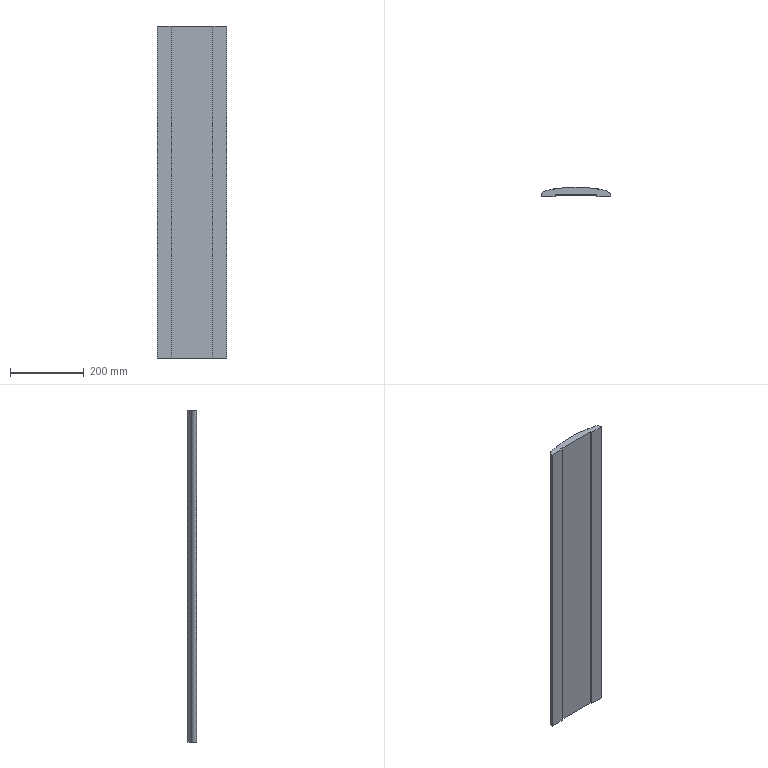Part | SolidWorks | features Extrusion 1, Fillet 1 | 1 solid | 31 faces | box 188.037 x 25 x 900 mm | volume 2969495 mm3 | cylinder 24 | plane 7 | commonest cylinder face diameters 0.2 x8 0.6 x6 661 x5 28 x3 0.4 x2
STEP:
#1=CARTESIAN_POINT('',(-94.018,0.7177,450.));
#2=VERTEX_POINT('',#1);
#3=CARTESIAN_POINT('',(-94.012,0.2909,450.));
#4=VERTEX_POINT('',#3);
#5=CARTESIAN_POINT('',(-80.018,0.7177,450.));
#6=DIRECTION('',(0.,0.,1.));
#7=DIRECTION('',(1.,0.,0.));
#8=AXIS2_PLACEMENT_3D('',#5,#6,#7);
#9=CIRCLE('',#8,14.);
#10=EDGE_CURVE('',#2,#4,#9,.T.);
#11=ORIENTED_EDGE('',*,*,#10,.F.);
#12=CARTESIAN_POINT('',(-94.018,0.7177,-450.));
#13=VERTEX_POINT('',#12);
#14=CARTESIAN_POINT('',(-94.018,0.7177,450.));
#15=DIRECTION('',(0.,0.,-1.));
#16=VECTOR('',#15,1000.);
#17=LINE('',#14,#16);
#18=EDGE_CURVE('',#2,#13,#17,.T.);
#19=ORIENTED_EDGE('',*,*,#18,.T.);
#20=CARTESIAN_POINT('',(-94.012,0.2909,-450.));
#21=VERTEX_POINT('',#20);
#22=CARTESIAN_POINT('',(-80.018,0.7177,-450.));
#23=DIRECTION('',(0.,0.,1.));
#24=DIRECTION('',(1.,0.,0.));
#25=AXIS2_PLACEMENT_3D('',#22,#23,#24);
#26=CIRCLE('',#25,14.);
#27=EDGE_CURVE('',#13,#21,#26,.T.);
#28=ORIENTED_EDGE('',*,*,#27,.T.);
#29=CARTESIAN_POINT('',(-94.012,0.2909,450.));
#30=DIRECTION('',(0.,0.,1.));
#31=VECTOR('',#30,1000.);
#32=LINE('',#29,#31);
#33=EDGE_CURVE('',#21,#4,#32,.T.);
#34=ORIENTED_EDGE('',*,*,#33,.T.);
#35=EDGE_LOOP('',(#11,#19,#28,#34));
#36=FACE_OUTER_BOUND('',#35,.T.);
#37=CARTESIAN_POINT('',(-80.018,0.7177,450.));
#38=DIRECTION('',(0.,0.,-1.));
#39=DIRECTION('',(-1.,0.,0.));
#40=AXIS2_PLACEMENT_3D('',#37,#38,#39);
#41=CYLINDRICAL_SURFACE('',#40,14.);
#42=ADVANCED_FACE('',(#36),#41,.T.);
#43=ORIENTED_EDGE('',*,*,#18,.F.);
#44=CARTESIAN_POINT('',(-83.558,14.263,450.));
#45=VERTEX_POINT('',#44);
#46=CARTESIAN_POINT('',(-80.018,0.7177,450.));
#47=DIRECTION('',(0.,0.,1.));
#48=DIRECTION('',(1.,0.,0.));
#49=AXIS2_PLACEMENT_3D('',#46,#47,#48);
#50=CIRCLE('',#49,14.);
#51=EDGE_CURVE('',#45,#2,#50,.T.);
#52=ORIENTED_EDGE('',*,*,#51,.F.);
#53=CARTESIAN_POINT('',(-83.558,14.263,-450.));
#54=VERTEX_POINT('',#53);
#55=CARTESIAN_POINT('',(-83.558,14.263,450.));
#56=DIRECTION('',(0.,0.,-1.));
#57=VECTOR('',#56,1000.);
#58=LINE('',#55,#57);
#59=EDGE_CURVE('',#45,#54,#58,.T.);
#60=ORIENTED_EDGE('',*,*,#59,.T.);
#61=CARTESIAN_POINT('',(-80.018,0.7177,-450.));
#62=DIRECTION('',(0.,0.,1.));
#63=DIRECTION('',(1.,0.,0.));
#64=AXIS2_PLACEMENT_3D('',#61,#62,#63);
#65=CIRCLE('',#64,14.);
#66=EDGE_CURVE('',#54,#13,#65,.T.);
#67=ORIENTED_EDGE('',*,*,#66,.T.);
#68=EDGE_LOOP('',(#43,#52,#60,#67));
#69=FACE_OUTER_BOUND('',#68,.T.);
#70=CARTESIAN_POINT('',(-80.018,0.7177,450.));
#71=DIRECTION('',(0.,0.,-1.));
#72=DIRECTION('',(-1.,0.,0.));
#73=AXIS2_PLACEMENT_3D('',#70,#71,#72);
#74=CYLINDRICAL_SURFACE('',#73,14.);
#75=ADVANCED_FACE('',(#69),#74,.T.);
#76=CARTESIAN_POINT('',(-93.712,0.,450.));
#77=VERTEX_POINT('',#76);
#78=CARTESIAN_POINT('',(-56.7,0.,450.));
#79=VERTEX_POINT('',#78);
#80=CARTESIAN_POINT('',(-56.7,0.,450.));
#81=DIRECTION('',(1.,0.,0.));
#82=VECTOR('',#81,1000.);
#83=LINE('',#80,#82);
#84=EDGE_CURVE('',#77,#79,#83,.T.);
#85=ORIENTED_EDGE('',*,*,#84,.F.);
#86=CARTESIAN_POINT('',(-93.712,0.,-450.));
#87=VERTEX_POINT('',#86);
#88=CARTESIAN_POINT('',(-93.712,0.,450.));
#89=DIRECTION('',(0.,0.,-1.));
#90=VECTOR('',#89,1000.);
#91=LINE('',#88,#90);
#92=EDGE_CURVE('',#77,#87,#91,.T.);
#93=ORIENTED_EDGE('',*,*,#92,.T.);
#94=CARTESIAN_POINT('',(-56.7,0.,-450.));
#95=VERTEX_POINT('',#94);
#96=CARTESIAN_POINT('',(-56.7,0.,-450.));
#97=DIRECTION('',(1.,0.,0.));
#98=VECTOR('',#97,1000.);
#99=LINE('',#96,#98);
#100=EDGE_CURVE('',#87,#95,#99,.T.);
#101=ORIENTED_EDGE('',*,*,#100,.T.);
#102=CARTESIAN_POINT('',(-56.7,0.,450.));
#103=DIRECTION('',(0.,0.,-1.));
#104=VECTOR('',#103,1000.);
#105=LINE('',#102,#104);
#106=EDGE_CURVE('',#79,#95,#105,.T.);
#107=ORIENTED_EDGE('',*,*,#106,.F.);
#108=EDGE_LOOP('',(#85,#93,#101,#107));
#109=FACE_OUTER_BOUND('',#108,.T.);
#110=CARTESIAN_POINT('',(-56.7,0.,450.));
#111=DIRECTION('',(0.,1.,0.));
#112=DIRECTION('',(-1.,0.,0.));
#113=AXIS2_PLACEMENT_3D('',#110,#111,#112);
#114=PLANE('',#113);
#115=ADVANCED_FACE('',(#109),#114,.F.);
#116=CARTESIAN_POINT('',(-56.5,0.2,-450.));
#117=VERTEX_POINT('',#116);
#118=CARTESIAN_POINT('',(-56.7,0.2,-450.));
#119=DIRECTION('',(0.,0.,1.));
#120=DIRECTION('',(-1.,0.,0.));
#121=AXIS2_PLACEMENT_3D('',#118,#119,#120);
#122=CIRCLE('',#121,0.2);
#123=EDGE_CURVE('',#95,#117,#122,.T.);
#124=ORIENTED_EDGE('',*,*,#123,.T.);
#125=CARTESIAN_POINT('',(-56.5,0.2,450.));
#126=VERTEX_POINT('',#125);
#127=CARTESIAN_POINT('',(-56.5,0.2,450.));
#128=DIRECTION('',(0.,0.,-1.));
#129=VECTOR('',#128,1000.);
#130=LINE('',#127,#129);
#131=EDGE_CURVE('',#126,#117,#130,.T.);
#132=ORIENTED_EDGE('',*,*,#131,.F.);
#133=CARTESIAN_POINT('',(-56.7,0.2,450.));
#134=DIRECTION('',(0.,0.,1.));
#135=DIRECTION('',(-1.,0.,0.));
#136=AXIS2_PLACEMENT_3D('',#133,#134,#135);
#137=CIRCLE('',#136,0.2);
#138=EDGE_CURVE('',#79,#126,#137,.T.);
#139=ORIENTED_EDGE('',*,*,#138,.F.);
#140=ORIENTED_EDGE('',*,*,#106,.T.);
#141=EDGE_LOOP('',(#124,#132,#139,#140));
#142=FACE_OUTER_BOUND('',#141,.T.);
#143=CARTESIAN_POINT('',(-56.7,0.2,450.));
#144=DIRECTION('',(0.,0.,-1.));
#145=DIRECTION('',(-1.,0.,0.));
#146=AXIS2_PLACEMENT_3D('',#143,#144,#145);
#147=CYLINDRICAL_SURFACE('',#146,0.2);
#148=ADVANCED_FACE('',(#142),#147,.T.);
#149=CARTESIAN_POINT('',(-56.5,4.5,-450.));
#150=VERTEX_POINT('',#149);
#151=CARTESIAN_POINT('',(-56.5,0.2,-450.));
#152=DIRECTION('',(0.,1.,0.));
#153=VECTOR('',#152,1000.);
#154=LINE('',#151,#153);
#155=EDGE_CURVE('',#117,#150,#154,.T.);
#156=ORIENTED_EDGE('',*,*,#155,.T.);
#157=CARTESIAN_POINT('',(-56.5,4.5,450.));
#158=VERTEX_POINT('',#157);
#159=CARTESIAN_POINT('',(-56.5,4.5,450.));
#160=DIRECTION('',(0.,0.,-1.));
#161=VECTOR('',#160,1000.);
#162=LINE('',#159,#161);
#163=EDGE_CURVE('',#158,#150,#162,.T.);
#164=ORIENTED_EDGE('',*,*,#163,.F.);
#165=CARTESIAN_POINT('',(-56.5,0.2,450.));
#166=DIRECTION('',(0.,1.,0.));
#167=VECTOR('',#166,1000.);
#168=LINE('',#165,#167);
#169=EDGE_CURVE('',#126,#158,#168,.T.);
#170=ORIENTED_EDGE('',*,*,#169,.F.);
#171=ORIENTED_EDGE('',*,*,#131,.T.);
#172=EDGE_LOOP('',(#156,#164,#170,#171));
#173=FACE_OUTER_BOUND('',#172,.T.);
#174=CARTESIAN_POINT('',(-56.5,0.2,450.));
#175=DIRECTION('',(-1.,0.,0.));
#176=DIRECTION('',(0.,-1.,0.));
#177=AXIS2_PLACEMENT_3D('',#174,#175,#176);
#178=PLANE('',#177);
#179=ADVANCED_FACE('',(#173),#178,.F.);
#180=CARTESIAN_POINT('',(56.5,4.5,-450.));
#181=VERTEX_POINT('',#180);
#182=CARTESIAN_POINT('',(-56.5,4.5,-450.));
#183=DIRECTION('',(1.,0.,0.));
#184=VECTOR('',#183,1000.);
#185=LINE('',#182,#184);
#186=EDGE_CURVE('',#150,#181,#185,.T.);
#187=ORIENTED_EDGE('',*,*,#186,.T.);
#188=CARTESIAN_POINT('',(56.5,4.5,450.));
#189=VERTEX_POINT('',#188);
#190=CARTESIAN_POINT('',(56.5,4.5,450.));
#191=DIRECTION('',(0.,0.,-1.));
#192=VECTOR('',#191,1000.);
#193=LINE('',#190,#192);
#194=EDGE_CURVE('',#189,#181,#193,.T.);
#195=ORIENTED_EDGE('',*,*,#194,.F.);
#196=CARTESIAN_POINT('',(-56.5,4.5,450.));
#197=DIRECTION('',(1.,0.,0.));
#198=VECTOR('',#197,1000.);
#199=LINE('',#196,#198);
#200=EDGE_CURVE('',#158,#189,#199,.T.);
#201=ORIENTED_EDGE('',*,*,#200,.F.);
#202=ORIENTED_EDGE('',*,*,#163,.T.);
#203=EDGE_LOOP('',(#187,#195,#201,#202));
#204=FACE_OUTER_BOUND('',#203,.T.);
#205=CARTESIAN_POINT('',(-56.5,4.5,450.));
#206=DIRECTION('',(0.,1.,0.));
#207=DIRECTION('',(-1.,0.,0.));
#208=AXIS2_PLACEMENT_3D('',#205,#206,#207);
#209=PLANE('',#208);
#210=ADVANCED_FACE('',(#204),#209,.F.);
#211=CARTESIAN_POINT('',(56.5,0.2,-450.));
#212=VERTEX_POINT('',#211);
#213=CARTESIAN_POINT('',(56.5,0.2,-450.));
#214=DIRECTION('',(0.,-1.,0.));
#215=VECTOR('',#214,1000.);
#216=LINE('',#213,#215);
#217=EDGE_CURVE('',#181,#212,#216,.T.);
#218=ORIENTED_EDGE('',*,*,#217,.T.);
#219=CARTESIAN_POINT('',(56.5,0.2,450.));
#220=VERTEX_POINT('',#219);
#221=CARTESIAN_POINT('',(56.5,0.2,450.));
#222=DIRECTION('',(0.,0.,-1.));
#223=VECTOR('',#222,1000.);
#224=LINE('',#221,#223);
#225=EDGE_CURVE('',#220,#212,#224,.T.);
#226=ORIENTED_EDGE('',*,*,#225,.F.);
#227=CARTESIAN_POINT('',(56.5,0.2,450.));
#228=DIRECTION('',(0.,-1.,0.));
#229=VECTOR('',#228,1000.);
#230=LINE('',#227,#229);
#231=EDGE_CURVE('',#189,#220,#230,.T.);
#232=ORIENTED_EDGE('',*,*,#231,.F.);
#233=ORIENTED_EDGE('',*,*,#194,.T.);
#234=EDGE_LOOP('',(#218,#226,#232,#233));
#235=FACE_OUTER_BOUND('',#234,.T.);
#236=CARTESIAN_POINT('',(56.5,0.2,450.));
#237=DIRECTION('',(1.,0.,0.));
#238=DIRECTION('',(0.,1.,0.));
#239=AXIS2_PLACEMENT_3D('',#236,#237,#238);
#240=PLANE('',#239);
#241=ADVANCED_FACE('',(#235),#240,.F.);
#242=CARTESIAN_POINT('',(56.7,0.,-450.));
#243=VERTEX_POINT('',#242);
#244=CARTESIAN_POINT('',(56.7,0.2,-450.));
#245=DIRECTION('',(0.,0.,1.));
#246=DIRECTION('',(-1.,0.,0.));
#247=AXIS2_PLACEMENT_3D('',#244,#245,#246);
#248=CIRCLE('',#247,0.2);
#249=EDGE_CURVE('',#212,#243,#248,.T.);
#250=ORIENTED_EDGE('',*,*,#249,.T.);
#251=CARTESIAN_POINT('',(56.7,0.,450.));
#252=VERTEX_POINT('',#251);
#253=CARTESIAN_POINT('',(56.7,0.,450.));
#254=DIRECTION('',(0.,0.,-1.));
#255=VECTOR('',#254,1000.);
#256=LINE('',#253,#255);
#257=EDGE_CURVE('',#252,#243,#256,.T.);
#258=ORIENTED_EDGE('',*,*,#257,.F.);
#259=CARTESIAN_POINT('',(56.7,0.2,450.));
#260=DIRECTION('',(0.,0.,1.));
#261=DIRECTION('',(-1.,0.,0.));
#262=AXIS2_PLACEMENT_3D('',#259,#260,#261);
#263=CIRCLE('',#262,0.2);
#264=EDGE_CURVE('',#220,#252,#263,.T.);
#265=ORIENTED_EDGE('',*,*,#264,.F.);
#266=ORIENTED_EDGE('',*,*,#225,.T.);
#267=EDGE_LOOP('',(#250,#258,#265,#266));
#268=FACE_OUTER_BOUND('',#267,.T.);
#269=CARTESIAN_POINT('',(56.7,0.2,450.));
#270=DIRECTION('',(0.,0.,-1.));
#271=DIRECTION('',(-1.,0.,0.));
#272=AXIS2_PLACEMENT_3D('',#269,#270,#271);
#273=CYLINDRICAL_SURFACE('',#272,0.2);
#274=ADVANCED_FACE('',(#268),#273,.T.);
#275=CARTESIAN_POINT('',(93.712,0.,-450.));
#276=VERTEX_POINT('',#275);
#277=CARTESIAN_POINT('',(94.,0.,-450.));
#278=DIRECTION('',(1.,0.,0.));
#279=VECTOR('',#278,1000.);
#280=LINE('',#277,#279);
#281=EDGE_CURVE('',#243,#276,#280,.T.);
#282=ORIENTED_EDGE('',*,*,#281,.T.);
#283=CARTESIAN_POINT('',(93.712,0.,450.));
#284=VERTEX_POINT('',#283);
#285=CARTESIAN_POINT('',(93.712,0.,450.));
#286=DIRECTION('',(0.,0.,1.));
#287=VECTOR('',#286,1000.);
#288=LINE('',#285,#287);
#289=EDGE_CURVE('',#276,#284,#288,.T.);
#290=ORIENTED_EDGE('',*,*,#289,.T.);
#291=CARTESIAN_POINT('',(94.,0.,450.));
#292=DIRECTION('',(1.,0.,0.));
#293=VECTOR('',#292,1000.);
#294=LINE('',#291,#293);
#295=EDGE_CURVE('',#252,#284,#294,.T.);
#296=ORIENTED_EDGE('',*,*,#295,.F.);
#297=ORIENTED_EDGE('',*,*,#257,.T.);
#298=EDGE_LOOP('',(#282,#290,#296,#297));
#299=FACE_OUTER_BOUND('',#298,.T.);
#300=CARTESIAN_POINT('',(94.,0.,450.));
#301=DIRECTION('',(0.,1.,0.));
#302=DIRECTION('',(-1.,0.,0.));
#303=AXIS2_PLACEMENT_3D('',#300,#301,#302);
#304=PLANE('',#303);
#305=ADVANCED_FACE('',(#299),#304,.F.);
#306=CARTESIAN_POINT('',(94.012,0.2909,450.));
#307=VERTEX_POINT('',#306);
#308=CARTESIAN_POINT('',(83.558,14.263,450.));
#309=VERTEX_POINT('',#308);
#310=CARTESIAN_POINT('',(80.018,0.7177,450.));
#311=DIRECTION('',(0.,0.,1.));
#312=DIRECTION('',(-1.,0.,0.));
#313=AXIS2_PLACEMENT_3D('',#310,#311,#312);
#314=CIRCLE('',#313,14.);
#315=EDGE_CURVE('',#307,#309,#314,.T.);
#316=ORIENTED_EDGE('',*,*,#315,.F.);
#317=CARTESIAN_POINT('',(94.012,0.2909,-450.));
#318=VERTEX_POINT('',#317);
#319=CARTESIAN_POINT('',(94.012,0.2909,450.));
#320=DIRECTION('',(0.,0.,-1.));
#321=VECTOR('',#320,1000.);
#322=LINE('',#319,#321);
#323=EDGE_CURVE('',#307,#318,#322,.T.);
#324=ORIENTED_EDGE('',*,*,#323,.T.);
#325=CARTESIAN_POINT('',(83.558,14.263,-450.));
#326=VERTEX_POINT('',#325);
#327=CARTESIAN_POINT('',(80.018,0.7177,-450.));
#328=DIRECTION('',(0.,0.,1.));
#329=DIRECTION('',(-1.,0.,0.));
#330=AXIS2_PLACEMENT_3D('',#327,#328,#329);
#331=CIRCLE('',#330,14.);
#332=EDGE_CURVE('',#318,#326,#331,.T.);
#333=ORIENTED_EDGE('',*,*,#332,.T.);
#334=CARTESIAN_POINT('',(83.558,14.263,450.));
#335=DIRECTION('',(0.,0.,-1.));
#336=VECTOR('',#335,1000.);
#337=LINE('',#334,#336);
#338=EDGE_CURVE('',#309,#326,#337,.T.);
#339=ORIENTED_EDGE('',*,*,#338,.F.);
#340=EDGE_LOOP('',(#316,#324,#333,#339));
#341=FACE_OUTER_BOUND('',#340,.T.);
#342=CARTESIAN_POINT('',(80.018,0.7177,450.));
#343=DIRECTION('',(0.,0.,-1.));
#344=DIRECTION('',(-1.,0.,0.));
#345=AXIS2_PLACEMENT_3D('',#342,#343,#344);
#346=CYLINDRICAL_SURFACE('',#345,14.);
#347=ADVANCED_FACE('',(#341),#346,.T.);
#348=CARTESIAN_POINT('',(60.381,19.438,-450.));
#349=VERTEX_POINT('',#348);
#350=CARTESIAN_POINT('',(0.,-305.5,-450.));
#351=DIRECTION('',(0.,0.,1.));
#352=DIRECTION('',(1.,0.,0.));
#353=AXIS2_PLACEMENT_3D('',#350,#351,#352);
#354=CIRCLE('',#353,330.5);
#355=EDGE_CURVE('',#326,#349,#354,.T.);
#356=ORIENTED_EDGE('',*,*,#355,.T.);
#357=CARTESIAN_POINT('',(60.381,19.438,450.));
#358=VERTEX_POINT('',#357);
#359=CARTESIAN_POINT('',(60.381,19.438,450.));
#360=DIRECTION('',(0.,0.,-1.));
#361=VECTOR('',#360,1000.);
#362=LINE('',#359,#361);
#363=EDGE_CURVE('',#358,#349,#362,.T.);
#364=ORIENTED_EDGE('',*,*,#363,.F.);
#365=CARTESIAN_POINT('',(0.,-305.5,450.));
#366=DIRECTION('',(0.,0.,1.));
#367=DIRECTION('',(1.,0.,0.));
#368=AXIS2_PLACEMENT_3D('',#365,#366,#367);
#369=CIRCLE('',#368,330.5);
#370=EDGE_CURVE('',#309,#358,#369,.T.);
#371=ORIENTED_EDGE('',*,*,#370,.F.);
#372=ORIENTED_EDGE('',*,*,#338,.T.);
#373=EDGE_LOOP('',(#356,#364,#371,#372));
#374=FACE_OUTER_BOUND('',#373,.T.);
#375=CARTESIAN_POINT('',(0.,-305.5,450.));
#376=DIRECTION('',(0.,0.,-1.));
#377=DIRECTION('',(-1.,0.,0.));
#378=AXIS2_PLACEMENT_3D('',#375,#376,#377);
#379=CYLINDRICAL_SURFACE('',#378,330.5);
#380=ADVANCED_FACE('',(#374),#379,.T.);
#381=CARTESIAN_POINT('',(60.272,19.381,-450.));
#382=VERTEX_POINT('',#381);
#383=CARTESIAN_POINT('',(60.363,19.339,-450.));
#384=DIRECTION('',(0.,0.,1.));
#385=DIRECTION('',(1.,0.,0.));
#386=AXIS2_PLACEMENT_3D('',#383,#384,#385);
#387=CIRCLE('',#386,0.1);
#388=EDGE_CURVE('',#349,#382,#387,.T.);
#389=ORIENTED_EDGE('',*,*,#388,.T.);
#390=CARTESIAN_POINT('',(60.272,19.381,450.));
#391=VERTEX_POINT('',#390);
#392=CARTESIAN_POINT('',(60.272,19.381,450.));
#393=DIRECTION('',(0.,0.,-1.));
#394=VECTOR('',#393,1000.);
#395=LINE('',#392,#394);
#396=EDGE_CURVE('',#391,#382,#395,.T.);
#397=ORIENTED_EDGE('',*,*,#396,.F.);
#398=CARTESIAN_POINT('',(60.363,19.339,450.));
#399=DIRECTION('',(0.,0.,1.));
#400=DIRECTION('',(1.,0.,0.));
#401=AXIS2_PLACEMENT_3D('',#398,#399,#400);
#402=CIRCLE('',#401,0.1);
#403=EDGE_CURVE('',#358,#391,#402,.T.);
#404=ORIENTED_EDGE('',*,*,#403,.F.);
#405=ORIENTED_EDGE('',*,*,#363,.T.);
#406=EDGE_LOOP('',(#389,#397,#404,#405));
#407=FACE_OUTER_BOUND('',#406,.T.);
#408=CARTESIAN_POINT('',(60.363,19.339,450.));
#409=DIRECTION('',(0.,0.,-1.));
#410=DIRECTION('',(-1.,0.,0.));
#411=AXIS2_PLACEMENT_3D('',#408,#409,#410);
#412=CYLINDRICAL_SURFACE('',#411,0.1);
#413=ADVANCED_FACE('',(#407),#412,.T.);
#414=CARTESIAN_POINT('',(59.701,19.487,-450.));
#415=VERTEX_POINT('',#414);
#416=CARTESIAN_POINT('',(60.,19.508,-450.));
#417=DIRECTION('',(0.,0.,-1.));
#418=DIRECTION('',(-1.,0.,0.));
#419=AXIS2_PLACEMENT_3D('',#416,#417,#418);
#420=CIRCLE('',#419,0.3);
#421=EDGE_CURVE('',#382,#415,#420,.T.);
#422=ORIENTED_EDGE('',*,*,#421,.T.);
#423=CARTESIAN_POINT('',(59.701,19.487,450.));
#424=VERTEX_POINT('',#423);
#425=CARTESIAN_POINT('',(59.701,19.487,450.));
#426=DIRECTION('',(0.,0.,-1.));
#427=VECTOR('',#426,1000.);
#428=LINE('',#425,#427);
#429=EDGE_CURVE('',#424,#415,#428,.T.);
#430=ORIENTED_EDGE('',*,*,#429,.F.);
#431=CARTESIAN_POINT('',(60.,19.508,450.));
#432=DIRECTION('',(0.,0.,-1.));
#433=DIRECTION('',(-1.,0.,0.));
#434=AXIS2_PLACEMENT_3D('',#431,#432,#433);
#435=CIRCLE('',#434,0.3);
#436=EDGE_CURVE('',#391,#424,#435,.T.);
#437=ORIENTED_EDGE('',*,*,#436,.F.);
#438=ORIENTED_EDGE('',*,*,#396,.T.);
#439=EDGE_LOOP('',(#422,#430,#437,#438));
#440=FACE_OUTER_BOUND('',#439,.T.);
#441=CARTESIAN_POINT('',(60.,19.508,450.));
#442=DIRECTION('',(0.,0.,-1.));
#443=DIRECTION('',(-1.,0.,0.));
#444=AXIS2_PLACEMENT_3D('',#441,#442,#443);
#445=CYLINDRICAL_SURFACE('',#444,0.3);
#446=ADVANCED_FACE('',(#440),#445,.F.);
#447=CARTESIAN_POINT('',(59.619,19.578,-450.));
#448=VERTEX_POINT('',#447);
#449=CARTESIAN_POINT('',(59.601,19.48,-450.));
#450=DIRECTION('',(0.,0.,1.));
#451=DIRECTION('',(1.,0.,0.));
#452=AXIS2_PLACEMENT_3D('',#449,#450,#451);
#453=CIRCLE('',#452,0.1);
#454=EDGE_CURVE('',#415,#448,#453,.T.);
#455=ORIENTED_EDGE('',*,*,#454,.T.);
#456=CARTESIAN_POINT('',(59.619,19.578,450.));
#457=VERTEX_POINT('',#456);
#458=CARTESIAN_POINT('',(59.619,19.578,450.));
#459=DIRECTION('',(0.,0.,-1.));
#460=VECTOR('',#459,1000.);
#461=LINE('',#458,#460);
#462=EDGE_CURVE('',#457,#448,#461,.T.);
#463=ORIENTED_EDGE('',*,*,#462,.F.);
#464=CARTESIAN_POINT('',(59.601,19.48,450.));
#465=DIRECTION('',(0.,0.,1.));
#466=DIRECTION('',(1.,0.,0.));
#467=AXIS2_PLACEMENT_3D('',#464,#465,#466);
#468=CIRCLE('',#467,0.1);
#469=EDGE_CURVE('',#424,#457,#468,.T.);
#470=ORIENTED_EDGE('',*,*,#469,.F.);
#471=ORIENTED_EDGE('',*,*,#429,.T.);
#472=EDGE_LOOP('',(#455,#463,#470,#471));
#473=FACE_OUTER_BOUND('',#472,.T.);
#474=CARTESIAN_POINT('',(59.601,19.48,450.));
#475=DIRECTION('',(0.,0.,-1.));
#476=DIRECTION('',(-1.,0.,0.));
#477=AXIS2_PLACEMENT_3D('',#474,#475,#476);
#478=CYLINDRICAL_SURFACE('',#477,0.1);
#479=ADVANCED_FACE('',(#473),#478,.T.);
#480=CARTESIAN_POINT('',(59.381,19.622,-450.));
#481=VERTEX_POINT('',#480);
#482=CARTESIAN_POINT('',(0.,-305.5,-450.));
#483=DIRECTION('',(0.,0.,1.));
#484=DIRECTION('',(1.,0.,0.));
#485=AXIS2_PLACEMENT_3D('',#482,#483,#484);
#486=CIRCLE('',#485,330.5);
#487=EDGE_CURVE('',#448,#481,#486,.T.);
#488=ORIENTED_EDGE('',*,*,#487,.T.);
#489=CARTESIAN_POINT('',(59.381,19.622,450.));
#490=VERTEX_POINT('',#489);
#491=CARTESIAN_POINT('',(59.381,19.622,450.));
#492=DIRECTION('',(0.,0.,-1.));
#493=VECTOR('',#492,1000.);
#494=LINE('',#491,#493);
#495=EDGE_CURVE('',#490,#481,#494,.T.);
#496=ORIENTED_EDGE('',*,*,#495,.F.);
#497=CARTESIAN_POINT('',(0.,-305.5,450.));
#498=DIRECTION('',(0.,0.,1.));
#499=DIRECTION('',(1.,0.,0.));
#500=AXIS2_PLACEMENT_3D('',#497,#498,#499);
#501=CIRCLE('',#500,330.5);
#502=EDGE_CURVE('',#457,#490,#501,.T.);
#503=ORIENTED_EDGE('',*,*,#502,.F.);
#504=ORIENTED_EDGE('',*,*,#462,.T.);
#505=EDGE_LOOP('',(#488,#496,#503,#504));
#506=FACE_OUTER_BOUND('',#505,.T.);
#507=CARTESIAN_POINT('',(0.,-305.5,450.));
#508=DIRECTION('',(0.,0.,-1.));
#509=DIRECTION('',(-1.,0.,0.));
#510=AXIS2_PLACEMENT_3D('',#507,#508,#509);
#511=CYLINDRICAL_SURFACE('',#510,330.5);
#512=ADVANCED_FACE('',(#506),#511,.T.);
#513=CARTESIAN_POINT('',(59.272,19.565,-450.));
#514=VERTEX_POINT('',#513);
#515=CARTESIAN_POINT('',(59.363,19.523,-450.));
#516=DIRECTION('',(0.,0.,1.));
#517=DIRECTION('',(1.,0.,0.));
#518=AXIS2_PLACEMENT_3D('',#515,#516,#517);
#519=CIRCLE('',#518,0.1);
#520=EDGE_CURVE('',#481,#514,#519,.T.);
#521=ORIENTED_EDGE('',*,*,#520,.T.);
#522=CARTESIAN_POINT('',(59.272,19.565,450.));
#523=VERTEX_POINT('',#522);
#524=CARTESIAN_POINT('',(59.272,19.565,450.));
#525=DIRECTION('',(0.,0.,-1.));
#526=VECTOR('',#525,1000.);
#527=LINE('',#524,#526);
#528=EDGE_CURVE('',#523,#514,#527,.T.);
#529=ORIENTED_EDGE('',*,*,#528,.F.);
#530=CARTESIAN_POINT('',(59.363,19.523,450.));
#531=DIRECTION('',(0.,0.,1.));
#532=DIRECTION('',(1.,0.,0.));
#533=AXIS2_PLACEMENT_3D('',#530,#531,#532);
#534=CIRCLE('',#533,0.1);
#535=EDGE_CURVE('',#490,#523,#534,.T.);
#536=ORIENTED_EDGE('',*,*,#535,.F.);
#537=ORIENTED_EDGE('',*,*,#495,.T.);
#538=EDGE_LOOP('',(#521,#529,#536,#537));
#539=FACE_OUTER_BOUND('',#538,.T.);
#540=CARTESIAN_POINT('',(59.363,19.523,450.));
#541=DIRECTION('',(0.,0.,-1.));
#542=DIRECTION('',(-1.,0.,0.));
#543=AXIS2_PLACEMENT_3D('',#540,#541,#542);
#544=CYLINDRICAL_SURFACE('',#543,0.1);
#545=ADVANCED_FACE('',(#539),#544,.T.);
#546=CARTESIAN_POINT('',(58.701,19.669,-450.));
#547=VERTEX_POINT('',#546);
#548=CARTESIAN_POINT('',(59.,19.691,-450.));
#549=DIRECTION('',(0.,0.,-1.));
#550=DIRECTION('',(-1.,0.,0.));
#551=AXIS2_PLACEMENT_3D('',#548,#549,#550);
#552=CIRCLE('',#551,0.3);
#553=EDGE_CURVE('',#514,#547,#552,.T.);
#554=ORIENTED_EDGE('',*,*,#553,.T.);
#555=CARTESIAN_POINT('',(58.701,19.669,450.));
#556=VERTEX_POINT('',#555);
#557=CARTESIAN_POINT('',(58.701,19.669,450.));
#558=DIRECTION('',(0.,0.,-1.));
#559=VECTOR('',#558,1000.);
#560=LINE('',#557,#559);
#561=EDGE_CURVE('',#556,#547,#560,.T.);
#562=ORIENTED_EDGE('',*,*,#561,.F.);
#563=CARTESIAN_POINT('',(59.,19.691,450.));
#564=DIRECTION('',(0.,0.,-1.));
#565=DIRECTION('',(-1.,0.,0.));
#566=AXIS2_PLACEMENT_3D('',#563,#564,#565);
#567=CIRCLE('',#566,0.3);
#568=EDGE_CURVE('',#523,#556,#567,.T.);
#569=ORIENTED_EDGE('',*,*,#568,.F.);
#570=ORIENTED_EDGE('',*,*,#528,.T.);
#571=EDGE_LOOP('',(#554,#562,#569,#570));
#572=FACE_OUTER_BOUND('',#571,.T.);
#573=CARTESIAN_POINT('',(59.,19.691,450.));
#574=DIRECTION('',(0.,0.,-1.));
#575=DIRECTION('',(-1.,0.,0.));
#576=AXIS2_PLACEMENT_3D('',#573,#574,#575);
#577=CYLINDRICAL_SURFACE('',#576,0.3);
#578=ADVANCED_FACE('',(#572),#577,.F.);
#579=CARTESIAN_POINT('',(58.619,19.76,-450.));
#580=VERTEX_POINT('',#579);
#581=CARTESIAN_POINT('',(58.601,19.662,-450.));
#582=DIRECTION('',(0.,0.,1.));
#583=DIRECTION('',(-1.,0.,0.));
#584=AXIS2_PLACEMENT_3D('',#581,#582,#583);
#585=CIRCLE('',#584,0.1);
#586=EDGE_CURVE('',#547,#580,#585,.T.);
#587=ORIENTED_EDGE('',*,*,#586,.T.);
#588=CARTESIAN_POINT('',(58.619,19.76,450.));
#589=VERTEX_POINT('',#588);
#590=CARTESIAN_POINT('',(58.619,19.76,450.));
#591=DIRECTION('',(0.,0.,-1.));
#592=VECTOR('',#591,1000.);
#593=LINE('',#590,#592);
#594=EDGE_CURVE('',#589,#580,#593,.T.);
#595=ORIENTED_EDGE('',*,*,#594,.F.);
#596=CARTESIAN_POINT('',(58.601,19.662,450.));
#597=DIRECTION('',(0.,0.,1.));
#598=DIRECTION('',(-1.,0.,0.));
#599=AXIS2_PLACEMENT_3D('',#596,#597,#598);
#600=CIRCLE('',#599,0.1);
#601=EDGE_CURVE('',#556,#589,#600,.T.);
#602=ORIENTED_EDGE('',*,*,#601,.F.);
#603=ORIENTED_EDGE('',*,*,#561,.T.);
#604=EDGE_LOOP('',(#587,#595,#602,#603));
#605=FACE_OUTER_BOUND('',#604,.T.);
#606=CARTESIAN_POINT('',(58.601,19.662,450.));
#607=DIRECTION('',(0.,0.,-1.));
#608=DIRECTION('',(-1.,0.,0.));
#609=AXIS2_PLACEMENT_3D('',#606,#607,#608);
#610=CYLINDRICAL_SURFACE('',#609,0.1);
#611=ADVANCED_FACE('',(#605),#610,.T.);
#612=CARTESIAN_POINT('',(-58.619,19.76,-450.));
#613=VERTEX_POINT('',#612);
#614=CARTESIAN_POINT('',(0.,-305.5,-450.));
#615=DIRECTION('',(0.,0.,1.));
#616=DIRECTION('',(1.,0.,0.));
#617=AXIS2_PLACEMENT_3D('',#614,#615,#616);
#618=CIRCLE('',#617,330.5);
#619=EDGE_CURVE('',#580,#613,#618,.T.);
#620=ORIENTED_EDGE('',*,*,#619,.T.);
#621=CARTESIAN_POINT('',(-58.619,19.76,450.));
#622=VERTEX_POINT('',#621);
#623=CARTESIAN_POINT('',(-58.619,19.76,450.));
#624=DIRECTION('',(0.,0.,-1.));
#625=VECTOR('',#624,1000.);
#626=LINE('',#623,#625);
#627=EDGE_CURVE('',#622,#613,#626,.T.);
#628=ORIENTED_EDGE('',*,*,#627,.F.);
#629=CARTESIAN_POINT('',(0.,-305.5,450.));
#630=DIRECTION('',(0.,0.,1.));
#631=DIRECTION('',(1.,0.,0.));
#632=AXIS2_PLACEMENT_3D('',#629,#630,#631);
#633=CIRCLE('',#632,330.5);
#634=EDGE_CURVE('',#589,#622,#633,.T.);
#635=ORIENTED_EDGE('',*,*,#634,.F.);
#636=ORIENTED_EDGE('',*,*,#594,.T.);
#637=EDGE_LOOP('',(#620,#628,#635,#636));
#638=FACE_OUTER_BOUND('',#637,.T.);
#639=CARTESIAN_POINT('',(0.,-305.5,450.));
#640=DIRECTION('',(0.,0.,-1.));
#641=DIRECTION('',(-1.,0.,0.));
#642=AXIS2_PLACEMENT_3D('',#639,#640,#641);
#643=CYLINDRICAL_SURFACE('',#642,330.5);
#644=ADVANCED_FACE('',(#638),#643,.T.);
#645=CARTESIAN_POINT('',(-58.701,19.669,-450.));
#646=VERTEX_POINT('',#645);
#647=CARTESIAN_POINT('',(-58.601,19.662,-450.));
#648=DIRECTION('',(0.,0.,1.));
#649=DIRECTION('',(-1.,0.,0.));
#650=AXIS2_PLACEMENT_3D('',#647,#648,#649);
#651=CIRCLE('',#650,0.1);
#652=EDGE_CURVE('',#613,#646,#651,.T.);
#653=ORIENTED_EDGE('',*,*,#652,.T.);
#654=CARTESIAN_POINT('',(-58.701,19.669,450.));
#655=VERTEX_POINT('',#654);
#656=CARTESIAN_POINT('',(-58.701,19.669,450.));
#657=DIRECTION('',(0.,0.,-1.));
#658=VECTOR('',#657,1000.);
#659=LINE('',#656,#658);
#660=EDGE_CURVE('',#655,#646,#659,.T.);
#661=ORIENTED_EDGE('',*,*,#660,.F.);
#662=CARTESIAN_POINT('',(-58.601,19.662,450.));
#663=DIRECTION('',(0.,0.,1.));
#664=DIRECTION('',(-1.,0.,0.));
#665=AXIS2_PLACEMENT_3D('',#662,#663,#664);
#666=CIRCLE('',#665,0.1);
#667=EDGE_CURVE('',#622,#655,#666,.T.);
#668=ORIENTED_EDGE('',*,*,#667,.F.);
#669=ORIENTED_EDGE('',*,*,#627,.T.);
#670=EDGE_LOOP('',(#653,#661,#668,#669));
#671=FACE_OUTER_BOUND('',#670,.T.);
#672=CARTESIAN_POINT('',(-58.601,19.662,450.));
#673=DIRECTION('',(0.,0.,-1.));
#674=DIRECTION('',(-1.,0.,0.));
#675=AXIS2_PLACEMENT_3D('',#672,#673,#674);
#676=CYLINDRICAL_SURFACE('',#675,0.1);
#677=ADVANCED_FACE('',(#671),#676,.T.);
#678=CARTESIAN_POINT('',(-59.272,19.565,-450.));
#679=VERTEX_POINT('',#678);
#680=CARTESIAN_POINT('',(-59.,19.691,-450.));
#681=DIRECTION('',(0.,0.,-1.));
#682=DIRECTION('',(1.,0.,0.));
#683=AXIS2_PLACEMENT_3D('',#680,#681,#682);
#684=CIRCLE('',#683,0.3);
#685=EDGE_CURVE('',#646,#679,#684,.T.);
#686=ORIENTED_EDGE('',*,*,#685,.T.);
#687=CARTESIAN_POINT('',(-59.272,19.565,450.));
#688=VERTEX_POINT('',#687);
#689=CARTESIAN_POINT('',(-59.272,19.565,450.));
#690=DIRECTION('',(0.,0.,-1.));
#691=VECTOR('',#690,1000.);
#692=LINE('',#689,#691);
#693=EDGE_CURVE('',#688,#679,#692,.T.);
#694=ORIENTED_EDGE('',*,*,#693,.F.);
#695=CARTESIAN_POINT('',(-59.,19.691,450.));
#696=DIRECTION('',(0.,0.,-1.));
#697=DIRECTION('',(1.,0.,0.));
#698=AXIS2_PLACEMENT_3D('',#695,#696,#697);
#699=CIRCLE('',#698,0.3);
#700=EDGE_CURVE('',#655,#688,#699,.T.);
#701=ORIENTED_EDGE('',*,*,#700,.F.);
#702=ORIENTED_EDGE('',*,*,#660,.T.);
#703=EDGE_LOOP('',(#686,#694,#701,#702));
#704=FACE_OUTER_BOUND('',#703,.T.);
#705=CARTESIAN_POINT('',(-59.,19.691,450.));
#706=DIRECTION('',(0.,0.,-1.));
#707=DIRECTION('',(-1.,0.,0.));
#708=AXIS2_PLACEMENT_3D('',#705,#706,#707);
#709=CYLINDRICAL_SURFACE('',#708,0.3);
#710=ADVANCED_FACE('',(#704),#709,.F.);
#711=CARTESIAN_POINT('',(-59.381,19.622,-450.));
#712=VERTEX_POINT('',#711);
#713=CARTESIAN_POINT('',(-59.363,19.523,-450.));
#714=DIRECTION('',(0.,0.,1.));
#715=DIRECTION('',(1.,0.,0.));
#716=AXIS2_PLACEMENT_3D('',#713,#714,#715);
#717=CIRCLE('',#716,0.1);
#718=EDGE_CURVE('',#679,#712,#717,.T.);
#719=ORIENTED_EDGE('',*,*,#718,.T.);
#720=CARTESIAN_POINT('',(-59.381,19.622,450.));
#721=VERTEX_POINT('',#720);
#722=CARTESIAN_POINT('',(-59.381,19.622,450.));
#723=DIRECTION('',(0.,0.,-1.));
#724=VECTOR('',#723,1000.);
#725=LINE('',#722,#724);
#726=EDGE_CURVE('',#721,#712,#725,.T.);
#727=ORIENTED_EDGE('',*,*,#726,.F.);
#728=CARTESIAN_POINT('',(-59.363,19.523,450.));
#729=DIRECTION('',(0.,0.,1.));
#730=DIRECTION('',(1.,0.,0.));
#731=AXIS2_PLACEMENT_3D('',#728,#729,#730);
#732=CIRCLE('',#731,0.1);
#733=EDGE_CURVE('',#688,#721,#732,.T.);
#734=ORIENTED_EDGE('',*,*,#733,.F.);
#735=ORIENTED_EDGE('',*,*,#693,.T.);
#736=EDGE_LOOP('',(#719,#727,#734,#735));
#737=FACE_OUTER_BOUND('',#736,.T.);
#738=CARTESIAN_POINT('',(-59.363,19.523,450.));
#739=DIRECTION('',(0.,0.,-1.));
#740=DIRECTION('',(-1.,0.,0.));
#741=AXIS2_PLACEMENT_3D('',#738,#739,#740);
#742=CYLINDRICAL_SURFACE('',#741,0.1);
#743=ADVANCED_FACE('',(#737),#742,.T.);
#744=CARTESIAN_POINT('',(-59.619,19.578,-450.));
#745=VERTEX_POINT('',#744);
#746=CARTESIAN_POINT('',(0.,-305.5,-450.));
#747=DIRECTION('',(0.,0.,1.));
#748=DIRECTION('',(1.,0.,0.));
#749=AXIS2_PLACEMENT_3D('',#746,#747,#748);
#750=CIRCLE('',#749,330.5);
#751=EDGE_CURVE('',#712,#745,#750,.T.);
#752=ORIENTED_EDGE('',*,*,#751,.T.);
#753=CARTESIAN_POINT('',(-59.619,19.578,450.));
#754=VERTEX_POINT('',#753);
#755=CARTESIAN_POINT('',(-59.619,19.578,450.));
#756=DIRECTION('',(0.,0.,-1.));
#757=VECTOR('',#756,1000.);
#758=LINE('',#755,#757);
#759=EDGE_CURVE('',#754,#745,#758,.T.);
#760=ORIENTED_EDGE('',*,*,#759,.F.);
#761=CARTESIAN_POINT('',(0.,-305.5,450.));
#762=DIRECTION('',(0.,0.,1.));
#763=DIRECTION('',(1.,0.,0.));
#764=AXIS2_PLACEMENT_3D('',#761,#762,#763);
#765=CIRCLE('',#764,330.5);
#766=EDGE_CURVE('',#721,#754,#765,.T.);
#767=ORIENTED_EDGE('',*,*,#766,.F.);
#768=ORIENTED_EDGE('',*,*,#726,.T.);
#769=EDGE_LOOP('',(#752,#760,#767,#768));
#770=FACE_OUTER_BOUND('',#769,.T.);
#771=CARTESIAN_POINT('',(0.,-305.5,450.));
#772=DIRECTION('',(0.,0.,-1.));
#773=DIRECTION('',(-1.,0.,0.));
#774=AXIS2_PLACEMENT_3D('',#771,#772,#773);
#775=CYLINDRICAL_SURFACE('',#774,330.5);
#776=ADVANCED_FACE('',(#770),#775,.T.);
#777=CARTESIAN_POINT('',(-59.701,19.487,-450.));
#778=VERTEX_POINT('',#777);
#779=CARTESIAN_POINT('',(-59.601,19.48,-450.));
#780=DIRECTION('',(0.,0.,1.));
#781=DIRECTION('',(-1.,0.,0.));
#782=AXIS2_PLACEMENT_3D('',#779,#780,#781);
#783=CIRCLE('',#782,0.1);
#784=EDGE_CURVE('',#745,#778,#783,.T.);
#785=ORIENTED_EDGE('',*,*,#784,.T.);
#786=CARTESIAN_POINT('',(-59.701,19.487,450.));
#787=VERTEX_POINT('',#786);
#788=CARTESIAN_POINT('',(-59.701,19.487,450.));
#789=DIRECTION('',(0.,0.,-1.));
#790=VECTOR('',#789,1000.);
#791=LINE('',#788,#790);
#792=EDGE_CURVE('',#787,#778,#791,.T.);
#793=ORIENTED_EDGE('',*,*,#792,.F.);
#794=CARTESIAN_POINT('',(-59.601,19.48,450.));
#795=DIRECTION('',(0.,0.,1.));
#796=DIRECTION('',(-1.,0.,0.));
#797=AXIS2_PLACEMENT_3D('',#794,#795,#796);
#798=CIRCLE('',#797,0.1);
#799=EDGE_CURVE('',#754,#787,#798,.T.);
#800=ORIENTED_EDGE('',*,*,#799,.F.);
#801=ORIENTED_EDGE('',*,*,#759,.T.);
#802=EDGE_LOOP('',(#785,#793,#800,#801));
#803=FACE_OUTER_BOUND('',#802,.T.);
#804=CARTESIAN_POINT('',(-59.601,19.48,450.));
#805=DIRECTION('',(0.,0.,-1.));
#806=DIRECTION('',(-1.,0.,0.));
#807=AXIS2_PLACEMENT_3D('',#804,#805,#806);
#808=CYLINDRICAL_SURFACE('',#807,0.1);
#809=ADVANCED_FACE('',(#803),#808,.T.);
#810=CARTESIAN_POINT('',(-60.272,19.381,-450.));
#811=VERTEX_POINT('',#810);
#812=CARTESIAN_POINT('',(-60.,19.508,-450.));
#813=DIRECTION('',(0.,0.,-1.));
#814=DIRECTION('',(1.,0.,0.));
#815=AXIS2_PLACEMENT_3D('',#812,#813,#814);
#816=CIRCLE('',#815,0.3);
#817=EDGE_CURVE('',#778,#811,#816,.T.);
#818=ORIENTED_EDGE('',*,*,#817,.T.);
#819=CARTESIAN_POINT('',(-60.272,19.381,450.));
#820=VERTEX_POINT('',#819);
#821=CARTESIAN_POINT('',(-60.272,19.381,450.));
#822=DIRECTION('',(0.,0.,-1.));
#823=VECTOR('',#822,1000.);
#824=LINE('',#821,#823);
#825=EDGE_CURVE('',#820,#811,#824,.T.);
#826=ORIENTED_EDGE('',*,*,#825,.F.);
#827=CARTESIAN_POINT('',(-60.,19.508,450.));
#828=DIRECTION('',(0.,0.,-1.));
#829=DIRECTION('',(1.,0.,0.));
#830=AXIS2_PLACEMENT_3D('',#827,#828,#829);
#831=CIRCLE('',#830,0.3);
#832=EDGE_CURVE('',#787,#820,#831,.T.);
#833=ORIENTED_EDGE('',*,*,#832,.F.);
#834=ORIENTED_EDGE('',*,*,#792,.T.);
#835=EDGE_LOOP('',(#818,#826,#833,#834));
#836=FACE_OUTER_BOUND('',#835,.T.);
#837=CARTESIAN_POINT('',(-60.,19.508,450.));
#838=DIRECTION('',(0.,0.,-1.));
#839=DIRECTION('',(-1.,0.,0.));
#840=AXIS2_PLACEMENT_3D('',#837,#838,#839);
#841=CYLINDRICAL_SURFACE('',#840,0.3);
#842=ADVANCED_FACE('',(#836),#841,.F.);
#843=CARTESIAN_POINT('',(-60.381,19.438,-450.));
#844=VERTEX_POINT('',#843);
#845=CARTESIAN_POINT('',(-60.363,19.339,-450.));
#846=DIRECTION('',(0.,0.,1.));
#847=DIRECTION('',(1.,0.,0.));
#848=AXIS2_PLACEMENT_3D('',#845,#846,#847);
#849=CIRCLE('',#848,0.1);
#850=EDGE_CURVE('',#811,#844,#849,.T.);
#851=ORIENTED_EDGE('',*,*,#850,.T.);
#852=CARTESIAN_POINT('',(-60.381,19.438,450.));
#853=VERTEX_POINT('',#852);
#854=CARTESIAN_POINT('',(-60.381,19.438,450.));
#855=DIRECTION('',(0.,0.,-1.));
#856=VECTOR('',#855,1000.);
#857=LINE('',#854,#856);
#858=EDGE_CURVE('',#853,#844,#857,.T.);
#859=ORIENTED_EDGE('',*,*,#858,.F.);
#860=CARTESIAN_POINT('',(-60.363,19.339,450.));
#861=DIRECTION('',(0.,0.,1.));
#862=DIRECTION('',(1.,0.,0.));
#863=AXIS2_PLACEMENT_3D('',#860,#861,#862);
#864=CIRCLE('',#863,0.1);
#865=EDGE_CURVE('',#820,#853,#864,.T.);
#866=ORIENTED_EDGE('',*,*,#865,.F.);
#867=ORIENTED_EDGE('',*,*,#825,.T.);
#868=EDGE_LOOP('',(#851,#859,#866,#867));
#869=FACE_OUTER_BOUND('',#868,.T.);
#870=CARTESIAN_POINT('',(-60.363,19.339,450.));
#871=DIRECTION('',(0.,0.,-1.));
#872=DIRECTION('',(-1.,0.,0.));
#873=AXIS2_PLACEMENT_3D('',#870,#871,#872);
#874=CYLINDRICAL_SURFACE('',#873,0.1);
#875=ADVANCED_FACE('',(#869),#874,.T.);
#876=CARTESIAN_POINT('',(0.,-305.5,-450.));
#877=DIRECTION('',(0.,0.,1.));
#878=DIRECTION('',(1.,0.,0.));
#879=AXIS2_PLACEMENT_3D('',#876,#877,#878);
#880=CIRCLE('',#879,330.5);
#881=EDGE_CURVE('',#844,#54,#880,.T.);
#882=ORIENTED_EDGE('',*,*,#881,.T.);
#883=ORIENTED_EDGE('',*,*,#59,.F.);
#884=CARTESIAN_POINT('',(0.,-305.5,450.));
#885=DIRECTION('',(0.,0.,1.));
#886=DIRECTION('',(1.,0.,0.));
#887=AXIS2_PLACEMENT_3D('',#884,#885,#886);
#888=CIRCLE('',#887,330.5);
#889=EDGE_CURVE('',#853,#45,#888,.T.);
#890=ORIENTED_EDGE('',*,*,#889,.F.);
#891=ORIENTED_EDGE('',*,*,#858,.T.);
#892=EDGE_LOOP('',(#882,#883,#890,#891));
#893=FACE_OUTER_BOUND('',#892,.T.);
#894=CARTESIAN_POINT('',(0.,-305.5,450.));
#895=DIRECTION('',(0.,0.,-1.));
#896=DIRECTION('',(-1.,0.,0.));
#897=AXIS2_PLACEMENT_3D('',#894,#895,#896);
#898=CYLINDRICAL_SURFACE('',#897,330.5);
#899=ADVANCED_FACE('',(#893),#898,.T.);
#900=ORIENTED_EDGE('',*,*,#51,.T.);
#901=ORIENTED_EDGE('',*,*,#10,.T.);
#902=CARTESIAN_POINT('',(-93.712,0.3,450.));
#903=DIRECTION('',(0.,0.,1.));
#904=DIRECTION('',(1.,0.,0.));
#905=AXIS2_PLACEMENT_3D('',#902,#903,#904);
#906=CIRCLE('',#905,0.3);
#907=EDGE_CURVE('',#4,#77,#906,.T.);
#908=ORIENTED_EDGE('',*,*,#907,.T.);
#909=ORIENTED_EDGE('',*,*,#84,.T.);
#910=ORIENTED_EDGE('',*,*,#138,.T.);
#911=ORIENTED_EDGE('',*,*,#169,.T.);
#912=ORIENTED_EDGE('',*,*,#200,.T.);
#913=ORIENTED_EDGE('',*,*,#231,.T.);
#914=ORIENTED_EDGE('',*,*,#264,.T.);
#915=ORIENTED_EDGE('',*,*,#295,.T.);
#916=CARTESIAN_POINT('',(93.712,0.3,450.));
#917=DIRECTION('',(0.,0.,1.));
#918=DIRECTION('',(1.,0.,0.));
#919=AXIS2_PLACEMENT_3D('',#916,#917,#918);
#920=CIRCLE('',#919,0.3);
#921=EDGE_CURVE('',#284,#307,#920,.T.);
#922=ORIENTED_EDGE('',*,*,#921,.T.);
#923=ORIENTED_EDGE('',*,*,#315,.T.);
#924=ORIENTED_EDGE('',*,*,#370,.T.);
#925=ORIENTED_EDGE('',*,*,#403,.T.);
#926=ORIENTED_EDGE('',*,*,#436,.T.);
#927=ORIENTED_EDGE('',*,*,#469,.T.);
#928=ORIENTED_EDGE('',*,*,#502,.T.);
#929=ORIENTED_EDGE('',*,*,#535,.T.);
#930=ORIENTED_EDGE('',*,*,#568,.T.);
#931=ORIENTED_EDGE('',*,*,#601,.T.);
#932=ORIENTED_EDGE('',*,*,#634,.T.);
#933=ORIENTED_EDGE('',*,*,#667,.T.);
#934=ORIENTED_EDGE('',*,*,#700,.T.);
#935=ORIENTED_EDGE('',*,*,#733,.T.);
#936=ORIENTED_EDGE('',*,*,#766,.T.);
#937=ORIENTED_EDGE('',*,*,#799,.T.);
#938=ORIENTED_EDGE('',*,*,#832,.T.);
#939=ORIENTED_EDGE('',*,*,#865,.T.);
#940=ORIENTED_EDGE('',*,*,#889,.T.);
#941=EDGE_LOOP('',(#900,#901,#908,#909,#910,#911,#912,#913,#914,#915,#922,#923,#924,#925,#926,#927,#928,#929,#930,#931,#932,#933,#934,#935,#936,#937,#938,#939,#940));
#942=FACE_OUTER_BOUND('',#941,.T.);
#943=CARTESIAN_POINT('',(-80.018,0.7177,450.));
#944=DIRECTION('',(0.,0.,1.));
#945=DIRECTION('',(1.,0.,0.));
#946=AXIS2_PLACEMENT_3D('',#943,#944,#945);
#947=PLANE('',#946);
#948=ADVANCED_FACE('',(#942),#947,.T.);
#949=ORIENTED_EDGE('',*,*,#100,.F.);
#950=CARTESIAN_POINT('',(-93.712,0.3,-450.));
#951=DIRECTION('',(0.,0.,-1.));
#952=DIRECTION('',(1.,0.,0.));
#953=AXIS2_PLACEMENT_3D('',#950,#951,#952);
#954=CIRCLE('',#953,0.3);
#955=EDGE_CURVE('',#87,#21,#954,.T.);
#956=ORIENTED_EDGE('',*,*,#955,.T.);
#957=ORIENTED_EDGE('',*,*,#27,.F.);
#958=ORIENTED_EDGE('',*,*,#66,.F.);
#959=ORIENTED_EDGE('',*,*,#881,.F.);
#960=ORIENTED_EDGE('',*,*,#850,.F.);
#961=ORIENTED_EDGE('',*,*,#817,.F.);
#962=ORIENTED_EDGE('',*,*,#784,.F.);
#963=ORIENTED_EDGE('',*,*,#751,.F.);
#964=ORIENTED_EDGE('',*,*,#718,.F.);
#965=ORIENTED_EDGE('',*,*,#685,.F.);
#966=ORIENTED_EDGE('',*,*,#652,.F.);
#967=ORIENTED_EDGE('',*,*,#619,.F.);
#968=ORIENTED_EDGE('',*,*,#586,.F.);
#969=ORIENTED_EDGE('',*,*,#553,.F.);
#970=ORIENTED_EDGE('',*,*,#520,.F.);
#971=ORIENTED_EDGE('',*,*,#487,.F.);
#972=ORIENTED_EDGE('',*,*,#454,.F.);
#973=ORIENTED_EDGE('',*,*,#421,.F.);
#974=ORIENTED_EDGE('',*,*,#388,.F.);
#975=ORIENTED_EDGE('',*,*,#355,.F.);
#976=ORIENTED_EDGE('',*,*,#332,.F.);
#977=CARTESIAN_POINT('',(93.712,0.3,-450.));
#978=DIRECTION('',(0.,0.,-1.));
#979=DIRECTION('',(1.,0.,0.));
#980=AXIS2_PLACEMENT_3D('',#977,#978,#979);
#981=CIRCLE('',#980,0.3);
#982=EDGE_CURVE('',#318,#276,#981,.T.);
#983=ORIENTED_EDGE('',*,*,#982,.T.);
#984=ORIENTED_EDGE('',*,*,#281,.F.);
#985=ORIENTED_EDGE('',*,*,#249,.F.);
#986=ORIENTED_EDGE('',*,*,#217,.F.);
#987=ORIENTED_EDGE('',*,*,#186,.F.);
#988=ORIENTED_EDGE('',*,*,#155,.F.);
#989=ORIENTED_EDGE('',*,*,#123,.F.);
#990=EDGE_LOOP('',(#949,#956,#957,#958,#959,#960,#961,#962,#963,#964,#965,#966,#967,#968,#969,#970,#971,#972,#973,#974,#975,#976,#983,#984,#985,#986,#987,#988,#989));
#991=FACE_OUTER_BOUND('',#990,.T.);
#992=CARTESIAN_POINT('',(-80.018,0.7177,-450.));
#993=DIRECTION('',(0.,0.,1.));
#994=DIRECTION('',(1.,0.,0.));
#995=AXIS2_PLACEMENT_3D('',#992,#993,#994);
#996=PLANE('',#995);
#997=ADVANCED_FACE('',(#991),#996,.F.);
#998=ORIENTED_EDGE('',*,*,#907,.F.);
#999=ORIENTED_EDGE('',*,*,#33,.F.);
#1000=ORIENTED_EDGE('',*,*,#955,.F.);
#1001=ORIENTED_EDGE('',*,*,#92,.F.);
#1002=EDGE_LOOP('',(#998,#999,#1000,#1001));
#1003=FACE_OUTER_BOUND('',#1002,.T.);
#1004=CARTESIAN_POINT('',(-93.712,0.3,450.));
#1005=DIRECTION('',(0.,0.,-1.));
#1006=DIRECTION('',(-1.,0.,0.));
#1007=AXIS2_PLACEMENT_3D('',#1004,#1005,#1006);
#1008=CYLINDRICAL_SURFACE('',#1007,0.3);
#1009=ADVANCED_FACE('',(#1003),#1008,.T.);
#1010=ORIENTED_EDGE('',*,*,#921,.F.);
#1011=ORIENTED_EDGE('',*,*,#289,.F.);
#1012=ORIENTED_EDGE('',*,*,#982,.F.);
#1013=ORIENTED_EDGE('',*,*,#323,.F.);
#1014=EDGE_LOOP('',(#1010,#1011,#1012,#1013));
#1015=FACE_OUTER_BOUND('',#1014,.T.);
#1016=CARTESIAN_POINT('',(93.712,0.3,450.));
#1017=DIRECTION('',(0.,0.,-1.));
#1018=DIRECTION('',(-1.,0.,0.));
#1019=AXIS2_PLACEMENT_3D('',#1016,#1017,#1018);
#1020=CYLINDRICAL_SURFACE('',#1019,0.3);
#1021=ADVANCED_FACE('',(#1015),#1020,.T.);
#1022=CLOSED_SHELL('',(#42,#75,#115,#148,#179,#210,#241,#274,#305,#347,#380,#413,#446,#479,#512,#545,#578,#611,#644,#677,#710,#743,#776,#809,#842,#875,#899,#948,#997,#1009,#1021));
#1023=MANIFOLD_SOLID_BREP('',#1022);
#1024=CARTESIAN_POINT('',(0.,0.,0.));
#1025=DIRECTION('',(0.,0.,1.));
#1026=DIRECTION('',(1.,0.,0.));
#1027=AXIS2_PLACEMENT_3D('',#1024,#1025,#1026);
#1028=(LENGTH_UNIT()NAMED_UNIT(*)SI_UNIT(.MILLI.,.METRE.));
#1029=UNCERTAINTY_MEASURE_WITH_UNIT(LENGTH_MEASURE(0.00001),#1028,'','');
#1030=(NAMED_UNIT(*)PLANE_ANGLE_UNIT()SI_UNIT($,.RADIAN.));
#1031=(NAMED_UNIT(*)SI_UNIT($,.STERADIAN.)SOLID_ANGLE_UNIT());
#1032=(GEOMETRIC_REPRESENTATION_CONTEXT(3)GLOBAL_UNCERTAINTY_ASSIGNED_CONTEXT((#1029))GLOBAL_UNIT_ASSIGNED_CONTEXT((#1028,#1030,#1031))REPRESENTATION_CONTEXT('',''));
#1033=ADVANCED_BREP_SHAPE_REPRESENTATION('',(#1023,#1027),#1032);